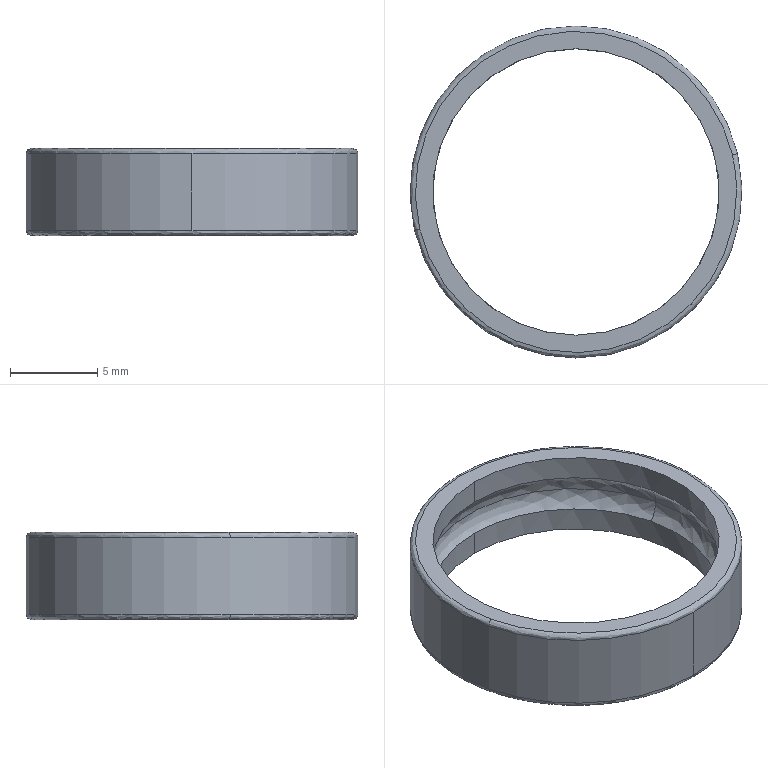Part | SolidWorks | features BaseBody 1 | 1 solid | 16 faces | box 19 x 19 x 5 mm | volume 321.706 mm3 | spline 8 | cylinder 6 | plane 2 | commonest cylinder face diameters 16.4 x4 19 x2
STEP:
#1=CARTESIAN_POINT('',(456.026,-100.404,305.244));
#2=VERTEX_POINT('',#1);
#3=CARTESIAN_POINT('',(465.27,-88.715,305.244));
#4=VERTEX_POINT('',#3);
#5=CARTESIAN_POINT('',(465.27,-98.215,305.244));
#6=DIRECTION('',(-0.000000004,0.00000001,-1.));
#7=DIRECTION('',(0.,1.,0.00000001));
#8=AXIS2_PLACEMENT_3D('',#5,#6,#7);
#9=CIRCLE('',#8,9.5);
#10=EDGE_CURVE('',#2,#4,#9,.T.);
#11=ORIENTED_EDGE('',*,*,#10,.F.);
#12=CARTESIAN_POINT('',(456.318,-100.335,305.544));
#13=VERTEX_POINT('',#12);
#14=CARTESIAN_POINT('',(456.318,-100.335,305.244));
#15=DIRECTION('',(-0.2304,0.9731,0.00000001));
#16=DIRECTION('',(-0.9731,-0.2304,0.000000002));
#17=AXIS2_PLACEMENT_3D('',#14,#15,#16);
#18=CIRCLE('',#17,0.3);
#19=EDGE_CURVE('',#2,#13,#18,.T.);
#20=ORIENTED_EDGE('',*,*,#19,.T.);
#21=CARTESIAN_POINT('',(474.223,-96.095,305.544));
#22=VERTEX_POINT('',#21);
#23=CARTESIAN_POINT('',(456.318,-100.335,305.544));
#24=CARTESIAN_POINT('',(452.078,-82.43,305.544));
#25=CARTESIAN_POINT('',(469.983,-78.19,305.544));
#26=CARTESIAN_POINT('',(474.223,-96.095,305.544));
#27=(BOUNDED_CURVE()B_SPLINE_CURVE(3,(#23,#24,#25,#26),.UNSPECIFIED.,.F.,.F.)B_SPLINE_CURVE_WITH_KNOTS((4,4),(0.,1.),.UNSPECIFIED.)CURVE()GEOMETRIC_REPRESENTATION_ITEM()RATIONAL_B_SPLINE_CURVE((1.,0.3333,0.3333,1.))REPRESENTATION_ITEM(''));
#28=EDGE_CURVE('',#13,#22,#27,.T.);
#29=ORIENTED_EDGE('',*,*,#28,.T.);
#30=CARTESIAN_POINT('',(474.515,-96.026,305.244));
#31=VERTEX_POINT('',#30);
#32=CARTESIAN_POINT('',(474.223,-96.095,305.244));
#33=DIRECTION('',(0.2304,-0.9731,-0.00000001));
#34=DIRECTION('',(0.9731,0.2304,-0.000000002));
#35=AXIS2_PLACEMENT_3D('',#32,#33,#34);
#36=CIRCLE('',#35,0.3);
#37=EDGE_CURVE('',#31,#22,#36,.T.);
#38=ORIENTED_EDGE('',*,*,#37,.F.);
#39=CARTESIAN_POINT('',(465.27,-98.215,305.244));
#40=DIRECTION('',(-0.000000004,0.00000001,-1.));
#41=DIRECTION('',(0.,1.,0.00000001));
#42=AXIS2_PLACEMENT_3D('',#39,#40,#41);
#43=CIRCLE('',#42,9.5);
#44=EDGE_CURVE('',#4,#31,#43,.T.);
#45=ORIENTED_EDGE('',*,*,#44,.F.);
#46=EDGE_LOOP('',(#11,#20,#29,#38,#45));
#47=FACE_OUTER_BOUND('',#46,.T.);
#48=CARTESIAN_POINT('',(456.026,-100.404,305.244));
#49=CARTESIAN_POINT('',(451.648,-81.915,305.244));
#50=CARTESIAN_POINT('',(470.137,-77.537,305.244));
#51=CARTESIAN_POINT('',(474.515,-96.026,305.244));
#52=CARTESIAN_POINT('',(456.026,-100.404,305.42));
#53=CARTESIAN_POINT('',(451.648,-81.915,305.42));
#54=CARTESIAN_POINT('',(470.137,-77.537,305.42));
#55=CARTESIAN_POINT('',(474.515,-96.026,305.42));
#56=CARTESIAN_POINT('',(456.147,-100.375,305.544));
#57=CARTESIAN_POINT('',(451.826,-82.128,305.544));
#58=CARTESIAN_POINT('',(470.073,-77.808,305.544));
#59=CARTESIAN_POINT('',(474.394,-96.055,305.544));
#60=CARTESIAN_POINT('',(456.318,-100.335,305.544));
#61=CARTESIAN_POINT('',(452.078,-82.43,305.544));
#62=CARTESIAN_POINT('',(469.983,-78.19,305.544));
#63=CARTESIAN_POINT('',(474.223,-96.095,305.544));
#64=(BOUNDED_SURFACE()B_SPLINE_SURFACE(3,3,((#48,#49,#50,#51),(#52,#53,#54,#55),(#56,#57,#58,#59),(#60,#61,#62,#63)),.UNSPECIFIED.,.F.,.F.,.F.)B_SPLINE_SURFACE_WITH_KNOTS((4,4),(4,4),(0.,1.),(0.,1.),.UNSPECIFIED.)GEOMETRIC_REPRESENTATION_ITEM()RATIONAL_B_SPLINE_SURFACE(((1.,0.3333,0.3333,1.),(0.8047,0.2682,0.2682,0.8047),(0.8047,0.2682,0.2682,0.8047),(1.,0.3333,0.3333,1.)))REPRESENTATION_ITEM('')SURFACE());
#65=ADVANCED_FACE('',(#47),#64,.T.);
#66=CARTESIAN_POINT('',(474.223,-96.095,300.544));
#67=VERTEX_POINT('',#66);
#68=CARTESIAN_POINT('',(456.318,-100.335,300.544));
#69=VERTEX_POINT('',#68);
#70=CARTESIAN_POINT('',(474.223,-96.095,300.544));
#71=CARTESIAN_POINT('',(469.983,-78.19,300.544));
#72=CARTESIAN_POINT('',(452.078,-82.43,300.544));
#73=CARTESIAN_POINT('',(456.318,-100.335,300.544));
#74=(BOUNDED_CURVE()B_SPLINE_CURVE(3,(#70,#71,#72,#73),.UNSPECIFIED.,.F.,.F.)B_SPLINE_CURVE_WITH_KNOTS((4,4),(0.,1.),.UNSPECIFIED.)CURVE()GEOMETRIC_REPRESENTATION_ITEM()RATIONAL_B_SPLINE_CURVE((1.,0.3333,0.3333,1.))REPRESENTATION_ITEM(''));
#75=EDGE_CURVE('',#67,#69,#74,.T.);
#76=ORIENTED_EDGE('',*,*,#75,.T.);
#77=CARTESIAN_POINT('',(456.026,-100.404,300.844));
#78=VERTEX_POINT('',#77);
#79=CARTESIAN_POINT('',(456.318,-100.335,300.844));
#80=DIRECTION('',(-0.2304,0.9731,0.00000001));
#81=DIRECTION('',(-0.9731,-0.2304,0.000000002));
#82=AXIS2_PLACEMENT_3D('',#79,#80,#81);
#83=CIRCLE('',#82,0.3);
#84=EDGE_CURVE('',#69,#78,#83,.T.);
#85=ORIENTED_EDGE('',*,*,#84,.T.);
#86=CARTESIAN_POINT('',(465.27,-88.715,300.844));
#87=VERTEX_POINT('',#86);
#88=CARTESIAN_POINT('',(465.27,-98.215,300.844));
#89=DIRECTION('',(0.000000004,-0.00000001,1.));
#90=DIRECTION('',(0.,1.,0.00000001));
#91=AXIS2_PLACEMENT_3D('',#88,#89,#90);
#92=CIRCLE('',#91,9.5);
#93=EDGE_CURVE('',#87,#78,#92,.T.);
#94=ORIENTED_EDGE('',*,*,#93,.F.);
#95=CARTESIAN_POINT('',(474.515,-96.026,300.844));
#96=VERTEX_POINT('',#95);
#97=CARTESIAN_POINT('',(465.27,-98.215,300.844));
#98=DIRECTION('',(0.000000004,-0.00000001,1.));
#99=DIRECTION('',(0.,1.,0.00000001));
#100=AXIS2_PLACEMENT_3D('',#97,#98,#99);
#101=CIRCLE('',#100,9.5);
#102=EDGE_CURVE('',#96,#87,#101,.T.);
#103=ORIENTED_EDGE('',*,*,#102,.F.);
#104=CARTESIAN_POINT('',(474.223,-96.095,300.844));
#105=DIRECTION('',(0.2304,-0.9731,-0.00000001));
#106=DIRECTION('',(0.9731,0.2304,-0.000000002));
#107=AXIS2_PLACEMENT_3D('',#104,#105,#106);
#108=CIRCLE('',#107,0.3);
#109=EDGE_CURVE('',#67,#96,#108,.T.);
#110=ORIENTED_EDGE('',*,*,#109,.F.);
#111=EDGE_LOOP('',(#76,#85,#94,#103,#110));
#112=FACE_OUTER_BOUND('',#111,.T.);
#113=CARTESIAN_POINT('',(456.318,-100.335,300.544));
#114=CARTESIAN_POINT('',(452.078,-82.43,300.544));
#115=CARTESIAN_POINT('',(469.983,-78.19,300.544));
#116=CARTESIAN_POINT('',(474.223,-96.095,300.544));
#117=CARTESIAN_POINT('',(456.147,-100.375,300.544));
#118=CARTESIAN_POINT('',(451.826,-82.128,300.544));
#119=CARTESIAN_POINT('',(470.073,-77.808,300.544));
#120=CARTESIAN_POINT('',(474.394,-96.055,300.544));
#121=CARTESIAN_POINT('',(456.026,-100.404,300.669));
#122=CARTESIAN_POINT('',(451.648,-81.915,300.669));
#123=CARTESIAN_POINT('',(470.137,-77.537,300.669));
#124=CARTESIAN_POINT('',(474.515,-96.026,300.669));
#125=CARTESIAN_POINT('',(456.026,-100.404,300.844));
#126=CARTESIAN_POINT('',(451.648,-81.915,300.844));
#127=CARTESIAN_POINT('',(470.137,-77.537,300.844));
#128=CARTESIAN_POINT('',(474.515,-96.026,300.844));
#129=(BOUNDED_SURFACE()B_SPLINE_SURFACE(3,3,((#113,#114,#115,#116),(#117,#118,#119,#120),(#121,#122,#123,#124),(#125,#126,#127,#128)),.UNSPECIFIED.,.F.,.F.,.F.)B_SPLINE_SURFACE_WITH_KNOTS((4,4),(4,4),(0.,1.),(0.,1.),.UNSPECIFIED.)GEOMETRIC_REPRESENTATION_ITEM()RATIONAL_B_SPLINE_SURFACE(((1.,0.3333,0.3333,1.),(0.8047,0.2682,0.2682,0.8047),(0.8047,0.2682,0.2682,0.8047),(1.,0.3333,0.3333,1.)))REPRESENTATION_ITEM('')SURFACE());
#130=ADVANCED_FACE('',(#112),#129,.T.);
#131=CARTESIAN_POINT('',(465.27,-106.415,301.949));
#132=VERTEX_POINT('',#131);
#133=CARTESIAN_POINT('',(457.291,-100.104,301.949));
#134=VERTEX_POINT('',#133);
#135=CARTESIAN_POINT('',(465.27,-98.215,301.949));
#136=DIRECTION('',(-0.000000004,0.00000001,-1.));
#137=DIRECTION('',(0.,1.,0.00000001));
#138=AXIS2_PLACEMENT_3D('',#135,#136,#137);
#139=CIRCLE('',#138,8.2);
#140=EDGE_CURVE('',#132,#134,#139,.T.);
#141=ORIENTED_EDGE('',*,*,#140,.T.);
#142=CARTESIAN_POINT('',(456.829,-100.214,303.044));
#143=VERTEX_POINT('',#142);
#144=CARTESIAN_POINT('',(458.288,-99.868,303.044));
#145=DIRECTION('',(-0.2304,0.9731,0.00000001));
#146=DIRECTION('',(-0.9731,-0.2304,0.000000002));
#147=AXIS2_PLACEMENT_3D('',#144,#145,#146);
#148=CIRCLE('',#147,1.5);
#149=EDGE_CURVE('',#134,#143,#148,.T.);
#150=ORIENTED_EDGE('',*,*,#149,.T.);
#151=CARTESIAN_POINT('',(473.712,-96.216,303.044));
#152=VERTEX_POINT('',#151);
#153=CARTESIAN_POINT('',(465.27,-98.215,303.044));
#154=DIRECTION('',(-0.000000004,0.00000001,-1.));
#155=DIRECTION('',(0.9731,0.2304,-0.000000002));
#156=AXIS2_PLACEMENT_3D('',#153,#154,#155);
#157=CIRCLE('',#156,8.675);
#158=EDGE_CURVE('',#152,#143,#157,.T.);
#159=ORIENTED_EDGE('',*,*,#158,.F.);
#160=CARTESIAN_POINT('',(473.25,-96.326,301.949));
#161=VERTEX_POINT('',#160);
#162=CARTESIAN_POINT('',(472.252,-96.562,303.044));
#163=DIRECTION('',(0.2304,-0.9731,-0.00000001));
#164=DIRECTION('',(0.9731,0.2304,-0.000000002));
#165=AXIS2_PLACEMENT_3D('',#162,#163,#164);
#166=CIRCLE('',#165,1.5);
#167=EDGE_CURVE('',#161,#152,#166,.T.);
#168=ORIENTED_EDGE('',*,*,#167,.F.);
#169=CARTESIAN_POINT('',(465.27,-98.215,301.949));
#170=DIRECTION('',(-0.000000004,0.00000001,-1.));
#171=DIRECTION('',(0.,1.,0.00000001));
#172=AXIS2_PLACEMENT_3D('',#169,#170,#171);
#173=CIRCLE('',#172,8.2);
#174=EDGE_CURVE('',#161,#132,#173,.T.);
#175=ORIENTED_EDGE('',*,*,#174,.T.);
#176=EDGE_LOOP('',(#141,#150,#159,#168,#175));
#177=FACE_OUTER_BOUND('',#176,.T.);
#178=CARTESIAN_POINT('',(473.25,-96.326,301.949));
#179=CARTESIAN_POINT('',(477.028,-112.285,301.949));
#180=CARTESIAN_POINT('',(461.069,-116.063,301.949));
#181=CARTESIAN_POINT('',(457.291,-100.104,301.949));
#182=CARTESIAN_POINT('',(473.549,-96.255,302.237));
#183=CARTESIAN_POINT('',(477.469,-112.812,302.237));
#184=CARTESIAN_POINT('',(460.912,-116.732,302.237));
#185=CARTESIAN_POINT('',(456.992,-100.175,302.237));
#186=CARTESIAN_POINT('',(473.712,-96.216,302.623));
#187=CARTESIAN_POINT('',(477.709,-113.1,302.623));
#188=CARTESIAN_POINT('',(460.826,-117.097,302.623));
#189=CARTESIAN_POINT('',(456.829,-100.214,302.623));
#190=CARTESIAN_POINT('',(473.712,-96.216,303.044));
#191=CARTESIAN_POINT('',(477.709,-113.1,303.044));
#192=CARTESIAN_POINT('',(460.826,-117.097,303.044));
#193=CARTESIAN_POINT('',(456.829,-100.214,303.044));
#194=(BOUNDED_SURFACE()B_SPLINE_SURFACE(3,3,((#178,#179,#180,#181),(#182,#183,#184,#185),(#186,#187,#188,#189),(#190,#191,#192,#193)),.UNSPECIFIED.,.F.,.F.,.F.)B_SPLINE_SURFACE_WITH_KNOTS((4,4),(4,4),(0.,1.),(0.,1.),.UNSPECIFIED.)GEOMETRIC_REPRESENTATION_ITEM()RATIONAL_B_SPLINE_SURFACE(((1.,0.3333,0.3333,1.),(0.9449,0.315,0.315,0.9449),(0.9449,0.315,0.315,0.9449),(1.,0.3333,0.3333,1.)))REPRESENTATION_ITEM('')SURFACE());
#195=ADVANCED_FACE('',(#177),#194,.F.);
#196=ORIENTED_EDGE('',*,*,#158,.T.);
#197=CARTESIAN_POINT('',(457.291,-100.104,304.139));
#198=VERTEX_POINT('',#197);
#199=CARTESIAN_POINT('',(458.288,-99.868,303.044));
#200=DIRECTION('',(-0.2304,0.9731,0.00000001));
#201=DIRECTION('',(-0.9731,-0.2304,0.000000002));
#202=AXIS2_PLACEMENT_3D('',#199,#200,#201);
#203=CIRCLE('',#202,1.5);
#204=EDGE_CURVE('',#143,#198,#203,.T.);
#205=ORIENTED_EDGE('',*,*,#204,.T.);
#206=CARTESIAN_POINT('',(465.27,-106.415,304.139));
#207=VERTEX_POINT('',#206);
#208=CARTESIAN_POINT('',(465.27,-98.215,304.139));
#209=DIRECTION('',(0.000000004,-0.00000001,1.));
#210=DIRECTION('',(0.,1.,0.00000001));
#211=AXIS2_PLACEMENT_3D('',#208,#209,#210);
#212=CIRCLE('',#211,8.2);
#213=EDGE_CURVE('',#198,#207,#212,.T.);
#214=ORIENTED_EDGE('',*,*,#213,.T.);
#215=CARTESIAN_POINT('',(473.25,-96.326,304.139));
#216=VERTEX_POINT('',#215);
#217=CARTESIAN_POINT('',(465.27,-98.215,304.139));
#218=DIRECTION('',(0.000000004,-0.00000001,1.));
#219=DIRECTION('',(0.,1.,0.00000001));
#220=AXIS2_PLACEMENT_3D('',#217,#218,#219);
#221=CIRCLE('',#220,8.2);
#222=EDGE_CURVE('',#207,#216,#221,.T.);
#223=ORIENTED_EDGE('',*,*,#222,.T.);
#224=CARTESIAN_POINT('',(472.252,-96.562,303.044));
#225=DIRECTION('',(0.2304,-0.9731,-0.00000001));
#226=DIRECTION('',(0.9731,0.2304,-0.000000002));
#227=AXIS2_PLACEMENT_3D('',#224,#225,#226);
#228=CIRCLE('',#227,1.5);
#229=EDGE_CURVE('',#152,#216,#228,.T.);
#230=ORIENTED_EDGE('',*,*,#229,.F.);
#231=EDGE_LOOP('',(#196,#205,#214,#223,#230));
#232=FACE_OUTER_BOUND('',#231,.T.);
#233=CARTESIAN_POINT('',(473.712,-96.216,303.044));
#234=CARTESIAN_POINT('',(477.709,-113.1,303.044));
#235=CARTESIAN_POINT('',(460.826,-117.097,303.044));
#236=CARTESIAN_POINT('',(456.829,-100.214,303.044));
#237=CARTESIAN_POINT('',(473.712,-96.216,303.465));
#238=CARTESIAN_POINT('',(477.709,-113.1,303.465));
#239=CARTESIAN_POINT('',(460.826,-117.097,303.465));
#240=CARTESIAN_POINT('',(456.829,-100.214,303.465));
#241=CARTESIAN_POINT('',(473.549,-96.255,303.852));
#242=CARTESIAN_POINT('',(477.469,-112.812,303.852));
#243=CARTESIAN_POINT('',(460.912,-116.732,303.852));
#244=CARTESIAN_POINT('',(456.992,-100.175,303.852));
#245=CARTESIAN_POINT('',(473.25,-96.326,304.139));
#246=CARTESIAN_POINT('',(477.028,-112.285,304.139));
#247=CARTESIAN_POINT('',(461.069,-116.063,304.139));
#248=CARTESIAN_POINT('',(457.291,-100.104,304.139));
#249=(BOUNDED_SURFACE()B_SPLINE_SURFACE(3,3,((#233,#234,#235,#236),(#237,#238,#239,#240),(#241,#242,#243,#244),(#245,#246,#247,#248)),.UNSPECIFIED.,.F.,.F.,.F.)B_SPLINE_SURFACE_WITH_KNOTS((4,4),(4,4),(0.,1.),(0.,1.),.UNSPECIFIED.)GEOMETRIC_REPRESENTATION_ITEM()RATIONAL_B_SPLINE_SURFACE(((1.,0.3333,0.3333,1.),(0.9449,0.315,0.315,0.9449),(0.9449,0.315,0.315,0.9449),(1.,0.3333,0.3333,1.)))REPRESENTATION_ITEM('')SURFACE());
#250=ADVANCED_FACE('',(#232),#249,.F.);
#251=ORIENTED_EDGE('',*,*,#44,.T.);
#252=CARTESIAN_POINT('',(465.27,-107.715,305.244));
#253=VERTEX_POINT('',#252);
#254=CARTESIAN_POINT('',(465.27,-98.215,305.244));
#255=DIRECTION('',(-0.000000004,0.00000001,-1.));
#256=DIRECTION('',(0.,1.,0.00000001));
#257=AXIS2_PLACEMENT_3D('',#254,#255,#256);
#258=CIRCLE('',#257,9.5);
#259=EDGE_CURVE('',#31,#253,#258,.T.);
#260=ORIENTED_EDGE('',*,*,#259,.T.);
#261=CARTESIAN_POINT('',(465.27,-107.715,300.844));
#262=VERTEX_POINT('',#261);
#263=CARTESIAN_POINT('',(465.27,-107.715,303.044));
#264=DIRECTION('',(-0.000000004,0.00000001,-1.));
#265=VECTOR('',#264,1000.);
#266=LINE('',#263,#265);
#267=EDGE_CURVE('',#253,#262,#266,.T.);
#268=ORIENTED_EDGE('',*,*,#267,.T.);
#269=CARTESIAN_POINT('',(465.27,-98.215,300.844));
#270=DIRECTION('',(0.000000004,-0.00000001,1.));
#271=DIRECTION('',(0.,1.,0.00000001));
#272=AXIS2_PLACEMENT_3D('',#269,#270,#271);
#273=CIRCLE('',#272,9.5);
#274=EDGE_CURVE('',#262,#96,#273,.T.);
#275=ORIENTED_EDGE('',*,*,#274,.T.);
#276=ORIENTED_EDGE('',*,*,#102,.T.);
#277=CARTESIAN_POINT('',(465.27,-88.715,303.044));
#278=DIRECTION('',(-0.000000004,0.00000001,-1.));
#279=VECTOR('',#278,1000.);
#280=LINE('',#277,#279);
#281=EDGE_CURVE('',#4,#87,#280,.T.);
#282=ORIENTED_EDGE('',*,*,#281,.F.);
#283=EDGE_LOOP('',(#251,#260,#268,#275,#276,#282));
#284=FACE_OUTER_BOUND('',#283,.T.);
#285=CARTESIAN_POINT('',(465.27,-98.215,303.044));
#286=DIRECTION('',(-0.000000004,0.00000001,-1.));
#287=DIRECTION('',(0.,1.,0.00000001));
#288=AXIS2_PLACEMENT_3D('',#285,#286,#287);
#289=CYLINDRICAL_SURFACE('',#288,9.5);
#290=ADVANCED_FACE('',(#284),#289,.T.);
#291=CARTESIAN_POINT('',(465.27,-106.415,305.544));
#292=VERTEX_POINT('',#291);
#293=CARTESIAN_POINT('',(465.27,-90.015,305.544));
#294=VERTEX_POINT('',#293);
#295=CARTESIAN_POINT('',(465.27,-98.215,305.544));
#296=DIRECTION('',(-0.000000004,0.00000001,-1.));
#297=DIRECTION('',(0.,1.,0.00000001));
#298=AXIS2_PLACEMENT_3D('',#295,#296,#297);
#299=CIRCLE('',#298,8.2);
#300=EDGE_CURVE('',#292,#294,#299,.T.);
#301=ORIENTED_EDGE('',*,*,#300,.F.);
#302=CARTESIAN_POINT('',(465.27,-106.415,304.842));
#303=DIRECTION('',(-0.000000004,0.00000001,-1.));
#304=VECTOR('',#303,1000.);
#305=LINE('',#302,#304);
#306=EDGE_CURVE('',#292,#207,#305,.T.);
#307=ORIENTED_EDGE('',*,*,#306,.T.);
#308=ORIENTED_EDGE('',*,*,#213,.F.);
#309=CARTESIAN_POINT('',(465.27,-90.015,304.139));
#310=VERTEX_POINT('',#309);
#311=CARTESIAN_POINT('',(465.27,-98.215,304.139));
#312=DIRECTION('',(0.000000004,-0.00000001,1.));
#313=DIRECTION('',(0.,1.,0.00000001));
#314=AXIS2_PLACEMENT_3D('',#311,#312,#313);
#315=CIRCLE('',#314,8.2);
#316=EDGE_CURVE('',#310,#198,#315,.T.);
#317=ORIENTED_EDGE('',*,*,#316,.F.);
#318=CARTESIAN_POINT('',(465.27,-90.015,304.842));
#319=DIRECTION('',(-0.000000004,0.00000001,-1.));
#320=VECTOR('',#319,1000.);
#321=LINE('',#318,#320);
#322=EDGE_CURVE('',#294,#310,#321,.T.);
#323=ORIENTED_EDGE('',*,*,#322,.F.);
#324=EDGE_LOOP('',(#301,#307,#308,#317,#323));
#325=FACE_OUTER_BOUND('',#324,.T.);
#326=CARTESIAN_POINT('',(465.27,-98.215,304.842));
#327=DIRECTION('',(-0.000000004,0.00000001,-1.));
#328=DIRECTION('',(0.,1.,0.00000001));
#329=AXIS2_PLACEMENT_3D('',#326,#327,#328);
#330=CYLINDRICAL_SURFACE('',#329,8.2);
#331=ADVANCED_FACE('',(#325),#330,.F.);
#332=ORIENTED_EDGE('',*,*,#140,.F.);
#333=CARTESIAN_POINT('',(465.27,-106.415,300.544));
#334=VERTEX_POINT('',#333);
#335=CARTESIAN_POINT('',(465.27,-106.415,301.247));
#336=DIRECTION('',(-0.000000004,0.00000001,-1.));
#337=VECTOR('',#336,1000.);
#338=LINE('',#335,#337);
#339=EDGE_CURVE('',#132,#334,#338,.T.);
#340=ORIENTED_EDGE('',*,*,#339,.T.);
#341=CARTESIAN_POINT('',(465.27,-90.015,300.544));
#342=VERTEX_POINT('',#341);
#343=CARTESIAN_POINT('',(465.27,-98.215,300.544));
#344=DIRECTION('',(0.000000004,-0.00000001,1.));
#345=DIRECTION('',(0.,1.,0.00000001));
#346=AXIS2_PLACEMENT_3D('',#343,#344,#345);
#347=CIRCLE('',#346,8.2);
#348=EDGE_CURVE('',#342,#334,#347,.T.);
#349=ORIENTED_EDGE('',*,*,#348,.F.);
#350=CARTESIAN_POINT('',(465.27,-90.015,301.949));
#351=VERTEX_POINT('',#350);
#352=CARTESIAN_POINT('',(465.27,-90.015,301.247));
#353=DIRECTION('',(-0.000000004,0.00000001,-1.));
#354=VECTOR('',#353,1000.);
#355=LINE('',#352,#354);
#356=EDGE_CURVE('',#351,#342,#355,.T.);
#357=ORIENTED_EDGE('',*,*,#356,.F.);
#358=CARTESIAN_POINT('',(465.27,-98.215,301.949));
#359=DIRECTION('',(-0.000000004,0.00000001,-1.));
#360=DIRECTION('',(0.,1.,0.00000001));
#361=AXIS2_PLACEMENT_3D('',#358,#359,#360);
#362=CIRCLE('',#361,8.2);
#363=EDGE_CURVE('',#134,#351,#362,.T.);
#364=ORIENTED_EDGE('',*,*,#363,.F.);
#365=EDGE_LOOP('',(#332,#340,#349,#357,#364));
#366=FACE_OUTER_BOUND('',#365,.T.);
#367=CARTESIAN_POINT('',(465.27,-98.215,301.247));
#368=DIRECTION('',(-0.000000004,0.00000001,-1.));
#369=DIRECTION('',(0.,1.,0.00000001));
#370=AXIS2_PLACEMENT_3D('',#367,#368,#369);
#371=CYLINDRICAL_SURFACE('',#370,8.2);
#372=ADVANCED_FACE('',(#366),#371,.F.);
#373=ORIENTED_EDGE('',*,*,#204,.F.);
#374=CARTESIAN_POINT('',(465.27,-98.215,303.044));
#375=DIRECTION('',(-0.000000004,0.00000001,-1.));
#376=DIRECTION('',(0.9731,0.2304,-0.000000002));
#377=AXIS2_PLACEMENT_3D('',#374,#375,#376);
#378=CIRCLE('',#377,8.675);
#379=EDGE_CURVE('',#143,#152,#378,.T.);
#380=ORIENTED_EDGE('',*,*,#379,.T.);
#381=ORIENTED_EDGE('',*,*,#229,.T.);
#382=CARTESIAN_POINT('',(465.27,-98.215,304.139));
#383=DIRECTION('',(0.000000004,-0.00000001,1.));
#384=DIRECTION('',(0.,1.,0.00000001));
#385=AXIS2_PLACEMENT_3D('',#382,#383,#384);
#386=CIRCLE('',#385,8.2);
#387=EDGE_CURVE('',#216,#310,#386,.T.);
#388=ORIENTED_EDGE('',*,*,#387,.T.);
#389=ORIENTED_EDGE('',*,*,#316,.T.);
#390=EDGE_LOOP('',(#373,#380,#381,#388,#389));
#391=FACE_OUTER_BOUND('',#390,.T.);
#392=CARTESIAN_POINT('',(456.829,-100.214,303.044));
#393=CARTESIAN_POINT('',(452.831,-83.33,303.044));
#394=CARTESIAN_POINT('',(469.715,-79.333,303.044));
#395=CARTESIAN_POINT('',(473.712,-96.216,303.044));
#396=CARTESIAN_POINT('',(456.829,-100.214,303.465));
#397=CARTESIAN_POINT('',(452.831,-83.33,303.465));
#398=CARTESIAN_POINT('',(469.715,-79.333,303.465));
#399=CARTESIAN_POINT('',(473.712,-96.216,303.465));
#400=CARTESIAN_POINT('',(456.992,-100.175,303.852));
#401=CARTESIAN_POINT('',(453.072,-83.618,303.852));
#402=CARTESIAN_POINT('',(469.629,-79.698,303.852));
#403=CARTESIAN_POINT('',(473.549,-96.255,303.852));
#404=CARTESIAN_POINT('',(457.291,-100.104,304.139));
#405=CARTESIAN_POINT('',(453.512,-84.145,304.139));
#406=CARTESIAN_POINT('',(469.471,-80.367,304.139));
#407=CARTESIAN_POINT('',(473.25,-96.326,304.139));
#408=(BOUNDED_SURFACE()B_SPLINE_SURFACE(3,3,((#392,#393,#394,#395),(#396,#397,#398,#399),(#400,#401,#402,#403),(#404,#405,#406,#407)),.UNSPECIFIED.,.F.,.F.,.F.)B_SPLINE_SURFACE_WITH_KNOTS((4,4),(4,4),(0.,1.),(0.,1.),.UNSPECIFIED.)GEOMETRIC_REPRESENTATION_ITEM()RATIONAL_B_SPLINE_SURFACE(((1.,0.3333,0.3333,1.),(0.9449,0.315,0.315,0.9449),(0.9449,0.315,0.315,0.9449),(1.,0.3333,0.3333,1.)))REPRESENTATION_ITEM('')SURFACE());
#409=ADVANCED_FACE('',(#391),#408,.F.);
#410=ORIENTED_EDGE('',*,*,#267,.F.);
#411=CARTESIAN_POINT('',(465.27,-98.215,305.244));
#412=DIRECTION('',(-0.000000004,0.00000001,-1.));
#413=DIRECTION('',(0.,1.,0.00000001));
#414=AXIS2_PLACEMENT_3D('',#411,#412,#413);
#415=CIRCLE('',#414,9.5);
#416=EDGE_CURVE('',#253,#2,#415,.T.);
#417=ORIENTED_EDGE('',*,*,#416,.T.);
#418=ORIENTED_EDGE('',*,*,#10,.T.);
#419=ORIENTED_EDGE('',*,*,#281,.T.);
#420=ORIENTED_EDGE('',*,*,#93,.T.);
#421=CARTESIAN_POINT('',(465.27,-98.215,300.844));
#422=DIRECTION('',(0.000000004,-0.00000001,1.));
#423=DIRECTION('',(0.,1.,0.00000001));
#424=AXIS2_PLACEMENT_3D('',#421,#422,#423);
#425=CIRCLE('',#424,9.5);
#426=EDGE_CURVE('',#78,#262,#425,.T.);
#427=ORIENTED_EDGE('',*,*,#426,.T.);
#428=EDGE_LOOP('',(#410,#417,#418,#419,#420,#427));
#429=FACE_OUTER_BOUND('',#428,.T.);
#430=CARTESIAN_POINT('',(465.27,-98.215,303.044));
#431=DIRECTION('',(-0.000000004,0.00000001,-1.));
#432=DIRECTION('',(0.,1.,0.00000001));
#433=AXIS2_PLACEMENT_3D('',#430,#431,#432);
#434=CYLINDRICAL_SURFACE('',#433,9.5);
#435=ADVANCED_FACE('',(#429),#434,.T.);
#436=ORIENTED_EDGE('',*,*,#19,.F.);
#437=ORIENTED_EDGE('',*,*,#416,.F.);
#438=ORIENTED_EDGE('',*,*,#259,.F.);
#439=ORIENTED_EDGE('',*,*,#37,.T.);
#440=CARTESIAN_POINT('',(456.318,-100.335,305.544));
#441=CARTESIAN_POINT('',(456.383,-100.608,305.544));
#442=CARTESIAN_POINT('',(456.498,-101.013,305.544));
#443=CARTESIAN_POINT('',(456.665,-101.474,305.544));
#444=CARTESIAN_POINT('',(456.756,-101.702,305.544));
#445=CARTESIAN_POINT('',(456.797,-101.799,305.544));
#446=CARTESIAN_POINT('',(456.825,-101.864,305.544));
#447=CARTESIAN_POINT('',(456.838,-101.894,305.544));
#448=CARTESIAN_POINT('',(456.973,-102.201,305.544));
#449=CARTESIAN_POINT('',(457.173,-102.6,305.544));
#450=CARTESIAN_POINT('',(457.439,-103.047,305.544));
#451=CARTESIAN_POINT('',(457.58,-103.265,305.544));
#452=CARTESIAN_POINT('',(457.642,-103.358,305.544));
#453=CARTESIAN_POINT('',(457.684,-103.42,305.544));
#454=CARTESIAN_POINT('',(457.704,-103.449,305.544));
#455=CARTESIAN_POINT('',(457.904,-103.736,305.544));
#456=CARTESIAN_POINT('',(458.189,-104.103,305.544));
#457=CARTESIAN_POINT('',(458.553,-104.504,305.544));
#458=CARTESIAN_POINT('',(458.715,-104.671,305.544));
#459=CARTESIAN_POINT('',(458.825,-104.78,305.544));
#460=CARTESIAN_POINT('',(458.879,-104.833,305.544));
#461=CARTESIAN_POINT('',(459.397,-105.325,305.544));
#462=CARTESIAN_POINT('',(459.898,-105.711,305.544));
#463=CARTESIAN_POINT('',(460.709,-106.211,305.544));
#464=CARTESIAN_POINT('',(461.125,-106.439,305.544));
#465=CARTESIAN_POINT('',(461.629,-106.666,305.544));
#466=CARTESIAN_POINT('',(461.849,-106.756,305.544));
#467=CARTESIAN_POINT('',(461.996,-106.813,305.544));
#468=CARTESIAN_POINT('',(462.072,-106.842,305.544));
#469=CARTESIAN_POINT('',(462.438,-106.974,305.544));
#470=CARTESIAN_POINT('',(462.882,-107.109,305.544));
#471=CARTESIAN_POINT('',(463.41,-107.227,305.544));
#472=CARTESIAN_POINT('',(463.677,-107.277,305.544));
#473=CARTESIAN_POINT('',(463.792,-107.296,305.544));
#474=CARTESIAN_POINT('',(463.869,-107.308,305.544));
#475=CARTESIAN_POINT('',(463.909,-107.314,305.544));
#476=CARTESIAN_POINT('',(464.241,-107.362,305.544));
#477=CARTESIAN_POINT('',(464.685,-107.405,305.544));
#478=CARTESIAN_POINT('',(465.204,-107.417,305.544));
#479=CARTESIAN_POINT('',(465.465,-107.413,305.544));
#480=CARTESIAN_POINT('',(465.576,-107.41,305.544));
#481=CARTESIAN_POINT('',(465.651,-107.407,305.544));
#482=CARTESIAN_POINT('',(465.69,-107.405,305.544));
#483=CARTESIAN_POINT('',(466.287,-107.376,305.544));
#484=CARTESIAN_POINT('',(466.843,-107.297,305.544));
#485=CARTESIAN_POINT('',(467.663,-107.103,305.544));
#486=CARTESIAN_POINT('',(468.068,-106.987,305.544));
#487=CARTESIAN_POINT('',(468.529,-106.82,305.544));
#488=CARTESIAN_POINT('',(468.757,-106.729,305.544));
#489=CARTESIAN_POINT('',(468.854,-106.688,305.544));
#490=CARTESIAN_POINT('',(468.919,-106.661,305.544));
#491=CARTESIAN_POINT('',(468.949,-106.647,305.544));
#492=CARTESIAN_POINT('',(469.256,-106.512,305.544));
#493=CARTESIAN_POINT('',(469.655,-106.313,305.544));
#494=CARTESIAN_POINT('',(470.102,-106.047,305.544));
#495=CARTESIAN_POINT('',(470.321,-105.905,305.544));
#496=CARTESIAN_POINT('',(470.413,-105.843,305.544));
#497=CARTESIAN_POINT('',(470.475,-105.801,305.544));
#498=CARTESIAN_POINT('',(470.505,-105.781,305.544));
#499=CARTESIAN_POINT('',(470.791,-105.581,305.544));
#500=CARTESIAN_POINT('',(471.158,-105.296,305.544));
#501=CARTESIAN_POINT('',(471.56,-104.933,305.544));
#502=CARTESIAN_POINT('',(471.726,-104.77,305.544));
#503=CARTESIAN_POINT('',(471.836,-104.66,305.544));
#504=CARTESIAN_POINT('',(471.889,-104.606,305.544));
#505=CARTESIAN_POINT('',(472.38,-104.088,305.544));
#506=CARTESIAN_POINT('',(472.766,-103.587,305.544));
#507=CARTESIAN_POINT('',(473.266,-102.776,305.544));
#508=CARTESIAN_POINT('',(473.494,-102.361,305.544));
#509=CARTESIAN_POINT('',(473.722,-101.856,305.544));
#510=CARTESIAN_POINT('',(473.811,-101.636,305.544));
#511=CARTESIAN_POINT('',(473.868,-101.489,305.544));
#512=CARTESIAN_POINT('',(473.897,-101.413,305.544));
#513=CARTESIAN_POINT('',(474.029,-101.047,305.544));
#514=CARTESIAN_POINT('',(474.164,-100.603,305.544));
#515=CARTESIAN_POINT('',(474.283,-100.075,305.544));
#516=CARTESIAN_POINT('',(474.332,-99.808,305.544));
#517=CARTESIAN_POINT('',(474.351,-99.693,305.544));
#518=CARTESIAN_POINT('',(474.363,-99.616,305.544));
#519=CARTESIAN_POINT('',(474.369,-99.576,305.544));
#520=CARTESIAN_POINT('',(474.417,-99.244,305.544));
#521=CARTESIAN_POINT('',(474.46,-98.801,305.544));
#522=CARTESIAN_POINT('',(474.472,-98.281,305.544));
#523=CARTESIAN_POINT('',(474.469,-98.02,305.544));
#524=CARTESIAN_POINT('',(474.465,-97.909,305.544));
#525=CARTESIAN_POINT('',(474.462,-97.834,305.544));
#526=CARTESIAN_POINT('',(474.461,-97.795,305.544));
#527=CARTESIAN_POINT('',(474.431,-97.198,305.544));
#528=CARTESIAN_POINT('',(474.352,-96.643,305.544));
#529=CARTESIAN_POINT('',(474.223,-96.095,305.544));
#530=B_SPLINE_CURVE_WITH_KNOTS('',3,(#440,#441,#442,#443,#444,#445,#446,#447,#448,#449,#450,#451,#452,#453,#454,#455,#456,#457,#458,#459,#460,#461,#462,#463,#464,#465,#466,#467,#468,#469,#470,#471,#472,#473,#474,#475,#476,#477,#478,#479,#480,#481,#482,#483,#484,#485,#486,#487,#488,#489,#490,#491,#492,#493,#494,#495,#496,#497,#498,#499,#500,#501,#502,#503,#504,#505,#506,#507,#508,#509,#510,#511,#512,#513,#514,#515,#516,#517,#518,#519,#520,#521,#522,#523,#524,#525,#526,#527,#528,#529),.UNSPECIFIED.,.F.,.F.,(4,1,1,1,2,2,1,1,1,2,2,1,1,2,2,2,1,1,2,2,1,1,1,2,2,1,1,1,2,2,2,1,1,1,2,2,1,1,1,2,2,1,1,2,2,2,1,1,2,2,1,1,1,2,2,1,1,1,2,2,4),(0.,0.03125,0.04688,0.05469,0.05859,0.0625,0.09375,0.1094,0.1172,0.1211,0.125,0.1562,0.1719,0.1797,0.1875,0.25,0.2812,0.2969,0.3047,0.3125,0.3437,0.3594,0.3672,0.3711,0.375,0.4062,0.4219,0.4297,0.4336,0.4375,0.5,0.5313,0.5469,0.5547,0.5586,0.5625,0.5938,0.6094,0.6172,0.6211,0.625,0.6563,0.6719,0.6797,0.6875,0.75,0.7813,0.7969,0.8047,0.8125,0.8438,0.8594,0.8672,0.8711,0.875,0.9063,0.9219,0.9297,0.9336,0.9375,1.),.UNSPECIFIED.);
#531=EDGE_CURVE('',#13,#22,#530,.T.);
#532=ORIENTED_EDGE('',*,*,#531,.F.);
#533=EDGE_LOOP('',(#436,#437,#438,#439,#532));
#534=FACE_OUTER_BOUND('',#533,.T.);
#535=CARTESIAN_POINT('',(474.515,-96.026,305.244));
#536=CARTESIAN_POINT('',(478.892,-114.515,305.244));
#537=CARTESIAN_POINT('',(460.403,-118.893,305.244));
#538=CARTESIAN_POINT('',(456.026,-100.404,305.244));
#539=CARTESIAN_POINT('',(474.515,-96.026,305.42));
#540=CARTESIAN_POINT('',(478.892,-114.515,305.42));
#541=CARTESIAN_POINT('',(460.403,-118.893,305.42));
#542=CARTESIAN_POINT('',(456.026,-100.404,305.42));
#543=CARTESIAN_POINT('',(474.394,-96.055,305.544));
#544=CARTESIAN_POINT('',(478.714,-114.302,305.544));
#545=CARTESIAN_POINT('',(460.467,-118.622,305.544));
#546=CARTESIAN_POINT('',(456.147,-100.375,305.544));
#547=CARTESIAN_POINT('',(474.223,-96.095,305.544));
#548=CARTESIAN_POINT('',(478.462,-114.,305.544));
#549=CARTESIAN_POINT('',(460.557,-118.24,305.544));
#550=CARTESIAN_POINT('',(456.318,-100.335,305.544));
#551=(BOUNDED_SURFACE()B_SPLINE_SURFACE(3,3,((#535,#536,#537,#538),(#539,#540,#541,#542),(#543,#544,#545,#546),(#547,#548,#549,#550)),.UNSPECIFIED.,.F.,.F.,.F.)B_SPLINE_SURFACE_WITH_KNOTS((4,4),(4,4),(0.,1.),(0.,1.),.UNSPECIFIED.)GEOMETRIC_REPRESENTATION_ITEM()RATIONAL_B_SPLINE_SURFACE(((1.,0.3333,0.3333,1.),(0.8047,0.2682,0.2682,0.8047),(0.8047,0.2682,0.2682,0.8047),(1.,0.3333,0.3333,1.)))REPRESENTATION_ITEM('')SURFACE());
#552=ADVANCED_FACE('',(#534),#551,.T.);
#553=ORIENTED_EDGE('',*,*,#84,.F.);
#554=CARTESIAN_POINT('',(456.318,-100.335,300.544));
#555=CARTESIAN_POINT('',(460.557,-118.24,300.544));
#556=CARTESIAN_POINT('',(478.462,-114.,300.544));
#557=CARTESIAN_POINT('',(474.223,-96.095,300.544));
#558=(BOUNDED_CURVE()B_SPLINE_CURVE(3,(#554,#555,#556,#557),.UNSPECIFIED.,.F.,.F.)B_SPLINE_CURVE_WITH_KNOTS((4,4),(0.,1.),.UNSPECIFIED.)CURVE()GEOMETRIC_REPRESENTATION_ITEM()RATIONAL_B_SPLINE_CURVE((1.,0.3333,0.3333,1.))REPRESENTATION_ITEM(''));
#559=EDGE_CURVE('',#69,#67,#558,.T.);
#560=ORIENTED_EDGE('',*,*,#559,.T.);
#561=ORIENTED_EDGE('',*,*,#109,.T.);
#562=ORIENTED_EDGE('',*,*,#274,.F.);
#563=ORIENTED_EDGE('',*,*,#426,.F.);
#564=EDGE_LOOP('',(#553,#560,#561,#562,#563));
#565=FACE_OUTER_BOUND('',#564,.T.);
#566=CARTESIAN_POINT('',(474.223,-96.095,300.544));
#567=CARTESIAN_POINT('',(478.462,-114.,300.544));
#568=CARTESIAN_POINT('',(460.557,-118.24,300.544));
#569=CARTESIAN_POINT('',(456.318,-100.335,300.544));
#570=CARTESIAN_POINT('',(474.394,-96.055,300.544));
#571=CARTESIAN_POINT('',(478.714,-114.302,300.544));
#572=CARTESIAN_POINT('',(460.467,-118.622,300.544));
#573=CARTESIAN_POINT('',(456.147,-100.375,300.544));
#574=CARTESIAN_POINT('',(474.515,-96.026,300.669));
#575=CARTESIAN_POINT('',(478.892,-114.515,300.669));
#576=CARTESIAN_POINT('',(460.403,-118.893,300.669));
#577=CARTESIAN_POINT('',(456.026,-100.404,300.669));
#578=CARTESIAN_POINT('',(474.515,-96.026,300.844));
#579=CARTESIAN_POINT('',(478.892,-114.515,300.844));
#580=CARTESIAN_POINT('',(460.403,-118.893,300.844));
#581=CARTESIAN_POINT('',(456.026,-100.404,300.844));
#582=(BOUNDED_SURFACE()B_SPLINE_SURFACE(3,3,((#566,#567,#568,#569),(#570,#571,#572,#573),(#574,#575,#576,#577),(#578,#579,#580,#581)),.UNSPECIFIED.,.F.,.F.,.F.)B_SPLINE_SURFACE_WITH_KNOTS((4,4),(4,4),(0.,1.),(0.,1.),.UNSPECIFIED.)GEOMETRIC_REPRESENTATION_ITEM()RATIONAL_B_SPLINE_SURFACE(((1.,0.3333,0.3333,1.),(0.8047,0.2682,0.2682,0.8047),(0.8047,0.2682,0.2682,0.8047),(1.,0.3333,0.3333,1.)))REPRESENTATION_ITEM('')SURFACE());
#583=ADVANCED_FACE('',(#565),#582,.T.);
#584=ORIENTED_EDGE('',*,*,#28,.F.);
#585=ORIENTED_EDGE('',*,*,#531,.T.);
#586=EDGE_LOOP('',(#584,#585));
#587=FACE_OUTER_BOUND('',#586,.T.);
#588=CARTESIAN_POINT('',(465.27,-98.215,305.544));
#589=DIRECTION('',(-0.000000004,0.00000001,-1.));
#590=DIRECTION('',(0.,1.,0.00000001));
#591=AXIS2_PLACEMENT_3D('',#588,#589,#590);
#592=CIRCLE('',#591,8.2);
#593=EDGE_CURVE('',#294,#292,#592,.T.);
#594=ORIENTED_EDGE('',*,*,#593,.T.);
#595=ORIENTED_EDGE('',*,*,#300,.T.);
#596=EDGE_LOOP('',(#594,#595));
#597=FACE_BOUND('',#596,.T.);
#598=CARTESIAN_POINT('',(473.736,-96.211,305.544));
#599=DIRECTION('',(0.000000004,-0.00000001,1.));
#600=DIRECTION('',(0.,-1.,-0.00000001));
#601=AXIS2_PLACEMENT_3D('',#598,#599,#600);
#602=PLANE('',#601);
#603=ADVANCED_FACE('',(#587,#597),#602,.T.);
#604=ORIENTED_EDGE('',*,*,#348,.T.);
#605=CARTESIAN_POINT('',(465.27,-98.215,300.544));
#606=DIRECTION('',(0.000000004,-0.00000001,1.));
#607=DIRECTION('',(0.,1.,0.00000001));
#608=AXIS2_PLACEMENT_3D('',#605,#606,#607);
#609=CIRCLE('',#608,8.2);
#610=EDGE_CURVE('',#334,#342,#609,.T.);
#611=ORIENTED_EDGE('',*,*,#610,.T.);
#612=EDGE_LOOP('',(#604,#611));
#613=FACE_BOUND('',#612,.T.);
#614=ORIENTED_EDGE('',*,*,#75,.F.);
#615=ORIENTED_EDGE('',*,*,#559,.F.);
#616=EDGE_LOOP('',(#614,#615));
#617=FACE_OUTER_BOUND('',#616,.T.);
#618=CARTESIAN_POINT('',(473.736,-96.211,300.544));
#619=DIRECTION('',(-0.000000004,0.00000001,-1.));
#620=DIRECTION('',(0.,1.,0.00000001));
#621=AXIS2_PLACEMENT_3D('',#618,#619,#620);
#622=PLANE('',#621);
#623=ADVANCED_FACE('',(#613,#617),#622,.T.);
#624=ORIENTED_EDGE('',*,*,#306,.F.);
#625=ORIENTED_EDGE('',*,*,#593,.F.);
#626=ORIENTED_EDGE('',*,*,#322,.T.);
#627=ORIENTED_EDGE('',*,*,#387,.F.);
#628=ORIENTED_EDGE('',*,*,#222,.F.);
#629=EDGE_LOOP('',(#624,#625,#626,#627,#628));
#630=FACE_OUTER_BOUND('',#629,.T.);
#631=CARTESIAN_POINT('',(465.27,-98.215,304.842));
#632=DIRECTION('',(-0.000000004,0.00000001,-1.));
#633=DIRECTION('',(0.,1.,0.00000001));
#634=AXIS2_PLACEMENT_3D('',#631,#632,#633);
#635=CYLINDRICAL_SURFACE('',#634,8.2);
#636=ADVANCED_FACE('',(#630),#635,.F.);
#637=ORIENTED_EDGE('',*,*,#339,.F.);
#638=ORIENTED_EDGE('',*,*,#174,.F.);
#639=CARTESIAN_POINT('',(465.27,-98.215,301.949));
#640=DIRECTION('',(-0.000000004,0.00000001,-1.));
#641=DIRECTION('',(0.,1.,0.00000001));
#642=AXIS2_PLACEMENT_3D('',#639,#640,#641);
#643=CIRCLE('',#642,8.2);
#644=EDGE_CURVE('',#351,#161,#643,.T.);
#645=ORIENTED_EDGE('',*,*,#644,.F.);
#646=ORIENTED_EDGE('',*,*,#356,.T.);
#647=ORIENTED_EDGE('',*,*,#610,.F.);
#648=EDGE_LOOP('',(#637,#638,#645,#646,#647));
#649=FACE_OUTER_BOUND('',#648,.T.);
#650=CARTESIAN_POINT('',(465.27,-98.215,301.247));
#651=DIRECTION('',(-0.000000004,0.00000001,-1.));
#652=DIRECTION('',(0.,1.,0.00000001));
#653=AXIS2_PLACEMENT_3D('',#650,#651,#652);
#654=CYLINDRICAL_SURFACE('',#653,8.2);
#655=ADVANCED_FACE('',(#649),#654,.F.);
#656=ORIENTED_EDGE('',*,*,#149,.F.);
#657=ORIENTED_EDGE('',*,*,#363,.T.);
#658=ORIENTED_EDGE('',*,*,#644,.T.);
#659=ORIENTED_EDGE('',*,*,#167,.T.);
#660=ORIENTED_EDGE('',*,*,#379,.F.);
#661=EDGE_LOOP('',(#656,#657,#658,#659,#660));
#662=FACE_OUTER_BOUND('',#661,.T.);
#663=CARTESIAN_POINT('',(457.291,-100.104,301.949));
#664=CARTESIAN_POINT('',(453.512,-84.145,301.949));
#665=CARTESIAN_POINT('',(469.471,-80.367,301.949));
#666=CARTESIAN_POINT('',(473.25,-96.326,301.949));
#667=CARTESIAN_POINT('',(456.992,-100.175,302.237));
#668=CARTESIAN_POINT('',(453.072,-83.618,302.237));
#669=CARTESIAN_POINT('',(469.629,-79.698,302.237));
#670=CARTESIAN_POINT('',(473.549,-96.255,302.237));
#671=CARTESIAN_POINT('',(456.829,-100.214,302.623));
#672=CARTESIAN_POINT('',(452.831,-83.33,302.623));
#673=CARTESIAN_POINT('',(469.715,-79.333,302.623));
#674=CARTESIAN_POINT('',(473.712,-96.216,302.623));
#675=CARTESIAN_POINT('',(456.829,-100.214,303.044));
#676=CARTESIAN_POINT('',(452.831,-83.33,303.044));
#677=CARTESIAN_POINT('',(469.715,-79.333,303.044));
#678=CARTESIAN_POINT('',(473.712,-96.216,303.044));
#679=(BOUNDED_SURFACE()B_SPLINE_SURFACE(3,3,((#663,#664,#665,#666),(#667,#668,#669,#670),(#671,#672,#673,#674),(#675,#676,#677,#678)),.UNSPECIFIED.,.F.,.F.,.F.)B_SPLINE_SURFACE_WITH_KNOTS((4,4),(4,4),(0.,1.),(0.,1.),.UNSPECIFIED.)GEOMETRIC_REPRESENTATION_ITEM()RATIONAL_B_SPLINE_SURFACE(((1.,0.3333,0.3333,1.),(0.9449,0.315,0.315,0.9449),(0.9449,0.315,0.315,0.9449),(1.,0.3333,0.3333,1.)))REPRESENTATION_ITEM('')SURFACE());
#680=ADVANCED_FACE('',(#662),#679,.F.);
#681=CLOSED_SHELL('',(#65,#130,#195,#250,#290,#331,#372,#409,#435,#552,#583,#603,#623,#636,#655,#680));
#682=MANIFOLD_SOLID_BREP('',#681);
#683=CARTESIAN_POINT('',(0.,0.,0.));
#684=DIRECTION('',(0.,0.,1.));
#685=DIRECTION('',(1.,0.,0.));
#686=AXIS2_PLACEMENT_3D('',#683,#684,#685);
#687=(LENGTH_UNIT()NAMED_UNIT(*)SI_UNIT(.MILLI.,.METRE.));
#688=UNCERTAINTY_MEASURE_WITH_UNIT(LENGTH_MEASURE(0.00001),#687,'','');
#689=(NAMED_UNIT(*)PLANE_ANGLE_UNIT()SI_UNIT($,.RADIAN.));
#690=(NAMED_UNIT(*)SI_UNIT($,.STERADIAN.)SOLID_ANGLE_UNIT());
#691=(GEOMETRIC_REPRESENTATION_CONTEXT(3)GLOBAL_UNCERTAINTY_ASSIGNED_CONTEXT((#688))GLOBAL_UNIT_ASSIGNED_CONTEXT((#687,#689,#690))REPRESENTATION_CONTEXT('',''));
#692=ADVANCED_BREP_SHAPE_REPRESENTATION('',(#682,#686),#691);